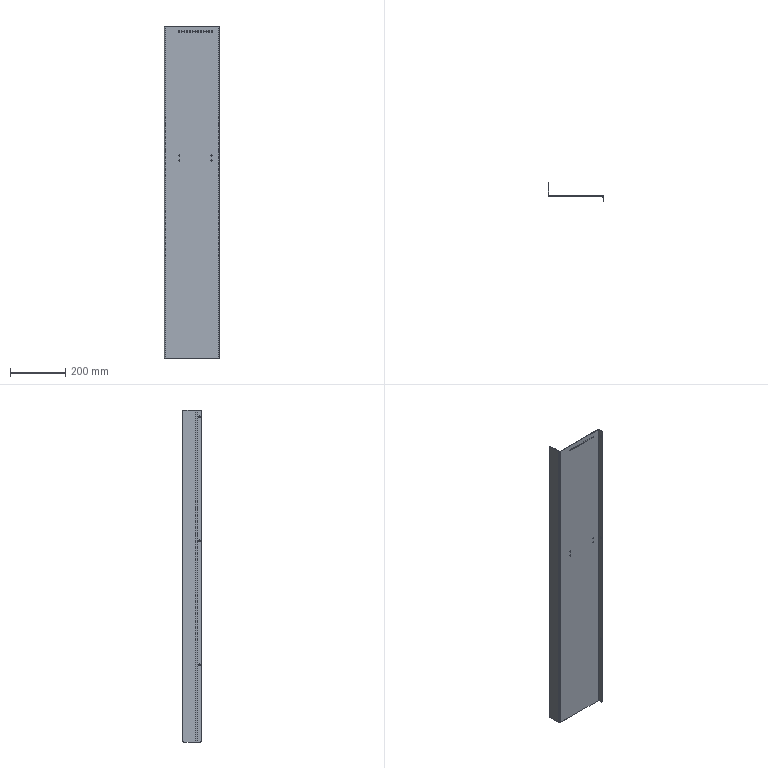Part | SolidWorks | features HoleWzd 3, Fillet 1, FlatPattern 1, ICE 1, SMBaseFlange 1, SheetMetal 1 | 1 solid | 62 faces | box 202 x 70 x 1205 mm | volume 643774 mm3 | cylinder 48 | plane 14 | commonest cylinder face diameters 4.2 x34 6.6 x6 10 x4 4 x2 8 x2